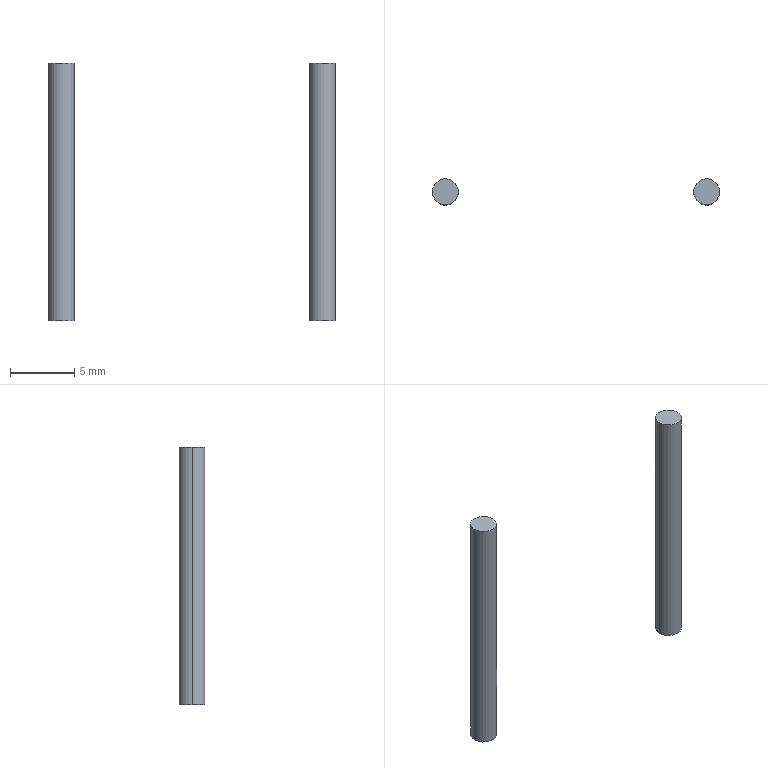Part | NX | features BREP 2 | 2 solids | 8 faces | box 22.254 x 2 x 20 mm | volume 125.664 mm3 | cylinder 4 | plane 4 | commonest cylinder face diameters 2 x4
STEP:
#1=CARTESIAN_POINT('',(10.939,112.404,-13.));
#2=VERTEX_POINT('',#1);
#3=CARTESIAN_POINT('',(8.939,112.404,-13.));
#4=VERTEX_POINT('',#3);
#5=CARTESIAN_POINT('',(9.939,112.404,-13.));
#6=DIRECTION('',(0.,0.,1.));
#7=DIRECTION('',(-1.,0.,0.));
#8=AXIS2_PLACEMENT_3D('',#5,#6,#7);
#9=CIRCLE('',#8,1.);
#10=EDGE_CURVE('',#2,#4,#9,.T.);
#11=ORIENTED_EDGE('',*,*,#10,.T.);
#12=CARTESIAN_POINT('',(8.939,112.404,7.));
#13=VERTEX_POINT('',#12);
#14=CARTESIAN_POINT('',(8.939,112.404,-8.828));
#15=DIRECTION('',(0.,0.,1.));
#16=VECTOR('',#15,1000.);
#17=LINE('',#14,#16);
#18=EDGE_CURVE('',#4,#13,#17,.T.);
#19=ORIENTED_EDGE('',*,*,#18,.T.);
#20=CARTESIAN_POINT('',(10.939,112.404,7.));
#21=VERTEX_POINT('',#20);
#22=CARTESIAN_POINT('',(9.939,112.404,7.));
#23=DIRECTION('',(0.,0.,1.));
#24=DIRECTION('',(1.,0.,0.));
#25=AXIS2_PLACEMENT_3D('',#22,#23,#24);
#26=CIRCLE('',#25,1.);
#27=EDGE_CURVE('',#21,#13,#26,.T.);
#28=ORIENTED_EDGE('',*,*,#27,.F.);
#29=CARTESIAN_POINT('',(10.939,112.404,-8.828));
#30=DIRECTION('',(0.,0.,1.));
#31=VECTOR('',#30,1000.);
#32=LINE('',#29,#31);
#33=EDGE_CURVE('',#2,#21,#32,.T.);
#34=ORIENTED_EDGE('',*,*,#33,.F.);
#35=EDGE_LOOP('',(#11,#19,#28,#34));
#36=FACE_BOUND('',#35,.T.);
#37=CARTESIAN_POINT('',(9.939,112.404,-8.828));
#38=DIRECTION('',(0.,0.,1.));
#39=DIRECTION('',(-1.,0.,0.));
#40=AXIS2_PLACEMENT_3D('',#37,#38,#39);
#41=CYLINDRICAL_SURFACE('',#40,1.);
#42=ADVANCED_FACE('',(#36),#41,.T.);
#43=ORIENTED_EDGE('',*,*,#10,.F.);
#44=CARTESIAN_POINT('',(9.939,112.404,-13.));
#45=DIRECTION('',(0.,0.,1.));
#46=DIRECTION('',(-1.,0.,0.));
#47=AXIS2_PLACEMENT_3D('',#44,#45,#46);
#48=CIRCLE('',#47,1.);
#49=EDGE_CURVE('',#4,#2,#48,.T.);
#50=ORIENTED_EDGE('',*,*,#49,.F.);
#51=EDGE_LOOP('',(#43,#50));
#52=FACE_BOUND('',#51,.T.);
#53=CARTESIAN_POINT('',(-31.187,83.404,-13.));
#54=DIRECTION('',(0.,0.,-1.));
#55=DIRECTION('',(0.,1.,0.));
#56=AXIS2_PLACEMENT_3D('',#53,#54,#55);
#57=PLANE('',#56);
#58=ADVANCED_FACE('',(#52),#57,.T.);
#59=ORIENTED_EDGE('',*,*,#27,.T.);
#60=CARTESIAN_POINT('',(9.939,112.404,7.));
#61=DIRECTION('',(0.,0.,1.));
#62=DIRECTION('',(1.,0.,0.));
#63=AXIS2_PLACEMENT_3D('',#60,#61,#62);
#64=CIRCLE('',#63,1.);
#65=EDGE_CURVE('',#13,#21,#64,.T.);
#66=ORIENTED_EDGE('',*,*,#65,.T.);
#67=EDGE_LOOP('',(#59,#66));
#68=FACE_BOUND('',#67,.T.);
#69=CARTESIAN_POINT('',(9.939,112.404,7.));
#70=DIRECTION('',(0.,0.,1.));
#71=DIRECTION('',(-1.,0.,0.));
#72=AXIS2_PLACEMENT_3D('',#69,#70,#71);
#73=PLANE('',#72);
#74=ADVANCED_FACE('',(#68),#73,.T.);
#75=ORIENTED_EDGE('',*,*,#18,.F.);
#76=ORIENTED_EDGE('',*,*,#49,.T.);
#77=ORIENTED_EDGE('',*,*,#33,.T.);
#78=ORIENTED_EDGE('',*,*,#65,.F.);
#79=EDGE_LOOP('',(#75,#76,#77,#78));
#80=FACE_BOUND('',#79,.T.);
#81=CARTESIAN_POINT('',(9.939,112.404,-8.828));
#82=DIRECTION('',(0.,0.,1.));
#83=DIRECTION('',(-1.,0.,0.));
#84=AXIS2_PLACEMENT_3D('',#81,#82,#83);
#85=CYLINDRICAL_SURFACE('',#84,1.);
#86=ADVANCED_FACE('',(#80),#85,.T.);
#87=CLOSED_SHELL('',(#42,#58,#74,#86));
#88=MANIFOLD_SOLID_BREP('',#87);
#89=CARTESIAN_POINT('',(-9.314,112.404,-13.));
#90=VERTEX_POINT('',#89);
#91=CARTESIAN_POINT('',(-11.314,112.404,-13.));
#92=VERTEX_POINT('',#91);
#93=CARTESIAN_POINT('',(-10.314,112.404,-13.));
#94=DIRECTION('',(0.,0.,1.));
#95=DIRECTION('',(-1.,0.,0.));
#96=AXIS2_PLACEMENT_3D('',#93,#94,#95);
#97=CIRCLE('',#96,1.);
#98=EDGE_CURVE('',#90,#92,#97,.T.);
#99=ORIENTED_EDGE('',*,*,#98,.T.);
#100=CARTESIAN_POINT('',(-11.314,112.404,7.));
#101=VERTEX_POINT('',#100);
#102=CARTESIAN_POINT('',(-11.314,112.404,-8.828));
#103=DIRECTION('',(0.,0.,1.));
#104=VECTOR('',#103,1000.);
#105=LINE('',#102,#104);
#106=EDGE_CURVE('',#92,#101,#105,.T.);
#107=ORIENTED_EDGE('',*,*,#106,.T.);
#108=CARTESIAN_POINT('',(-9.314,112.404,7.));
#109=VERTEX_POINT('',#108);
#110=CARTESIAN_POINT('',(-10.314,112.404,7.));
#111=DIRECTION('',(0.,0.,1.));
#112=DIRECTION('',(-1.,0.,0.));
#113=AXIS2_PLACEMENT_3D('',#110,#111,#112);
#114=CIRCLE('',#113,1.);
#115=EDGE_CURVE('',#109,#101,#114,.T.);
#116=ORIENTED_EDGE('',*,*,#115,.F.);
#117=CARTESIAN_POINT('',(-9.314,112.404,-8.828));
#118=DIRECTION('',(0.,0.,1.));
#119=VECTOR('',#118,1000.);
#120=LINE('',#117,#119);
#121=EDGE_CURVE('',#90,#109,#120,.T.);
#122=ORIENTED_EDGE('',*,*,#121,.F.);
#123=EDGE_LOOP('',(#99,#107,#116,#122));
#124=FACE_BOUND('',#123,.T.);
#125=CARTESIAN_POINT('',(-10.314,112.404,-8.828));
#126=DIRECTION('',(0.,0.,1.));
#127=DIRECTION('',(-1.,0.,0.));
#128=AXIS2_PLACEMENT_3D('',#125,#126,#127);
#129=CYLINDRICAL_SURFACE('',#128,1.);
#130=ADVANCED_FACE('',(#124),#129,.T.);
#131=ORIENTED_EDGE('',*,*,#98,.F.);
#132=CARTESIAN_POINT('',(-10.314,112.404,-13.));
#133=DIRECTION('',(0.,0.,1.));
#134=DIRECTION('',(-1.,0.,0.));
#135=AXIS2_PLACEMENT_3D('',#132,#133,#134);
#136=CIRCLE('',#135,1.);
#137=EDGE_CURVE('',#92,#90,#136,.T.);
#138=ORIENTED_EDGE('',*,*,#137,.F.);
#139=EDGE_LOOP('',(#131,#138));
#140=FACE_BOUND('',#139,.T.);
#141=CARTESIAN_POINT('',(-31.187,83.404,-13.));
#142=DIRECTION('',(0.,0.,-1.));
#143=DIRECTION('',(0.,1.,0.));
#144=AXIS2_PLACEMENT_3D('',#141,#142,#143);
#145=PLANE('',#144);
#146=ADVANCED_FACE('',(#140),#145,.T.);
#147=ORIENTED_EDGE('',*,*,#115,.T.);
#148=CARTESIAN_POINT('',(-10.314,112.404,7.));
#149=DIRECTION('',(0.,0.,1.));
#150=DIRECTION('',(-1.,0.,0.));
#151=AXIS2_PLACEMENT_3D('',#148,#149,#150);
#152=CIRCLE('',#151,1.);
#153=EDGE_CURVE('',#101,#109,#152,.T.);
#154=ORIENTED_EDGE('',*,*,#153,.T.);
#155=EDGE_LOOP('',(#147,#154));
#156=FACE_BOUND('',#155,.T.);
#157=CARTESIAN_POINT('',(-10.314,112.404,7.));
#158=DIRECTION('',(0.,0.,-1.));
#159=DIRECTION('',(0.,1.,0.));
#160=AXIS2_PLACEMENT_3D('',#157,#158,#159);
#161=PLANE('',#160);
#162=ADVANCED_FACE('',(#156),#161,.F.);
#163=ORIENTED_EDGE('',*,*,#106,.F.);
#164=ORIENTED_EDGE('',*,*,#137,.T.);
#165=ORIENTED_EDGE('',*,*,#121,.T.);
#166=ORIENTED_EDGE('',*,*,#153,.F.);
#167=EDGE_LOOP('',(#163,#164,#165,#166));
#168=FACE_BOUND('',#167,.T.);
#169=CARTESIAN_POINT('',(-10.314,112.404,-8.828));
#170=DIRECTION('',(0.,0.,1.));
#171=DIRECTION('',(-1.,0.,0.));
#172=AXIS2_PLACEMENT_3D('',#169,#170,#171);
#173=CYLINDRICAL_SURFACE('',#172,1.);
#174=ADVANCED_FACE('',(#168),#173,.T.);
#175=CLOSED_SHELL('',(#130,#146,#162,#174));
#176=MANIFOLD_SOLID_BREP('',#175);
#177=(LENGTH_UNIT()NAMED_UNIT(*)SI_UNIT(.MILLI.,.METRE.));
#178=UNCERTAINTY_MEASURE_WITH_UNIT(LENGTH_MEASURE(0.00001),#177,'','');
#179=(NAMED_UNIT(*)PLANE_ANGLE_UNIT()SI_UNIT($,.RADIAN.));
#180=(NAMED_UNIT(*)SI_UNIT($,.STERADIAN.)SOLID_ANGLE_UNIT());
#181=(GEOMETRIC_REPRESENTATION_CONTEXT(3)GLOBAL_UNCERTAINTY_ASSIGNED_CONTEXT((#178))GLOBAL_UNIT_ASSIGNED_CONTEXT((#177,#179,#180))REPRESENTATION_CONTEXT('',''));
#182=ADVANCED_BREP_SHAPE_REPRESENTATION('',(#88,#176),#181);